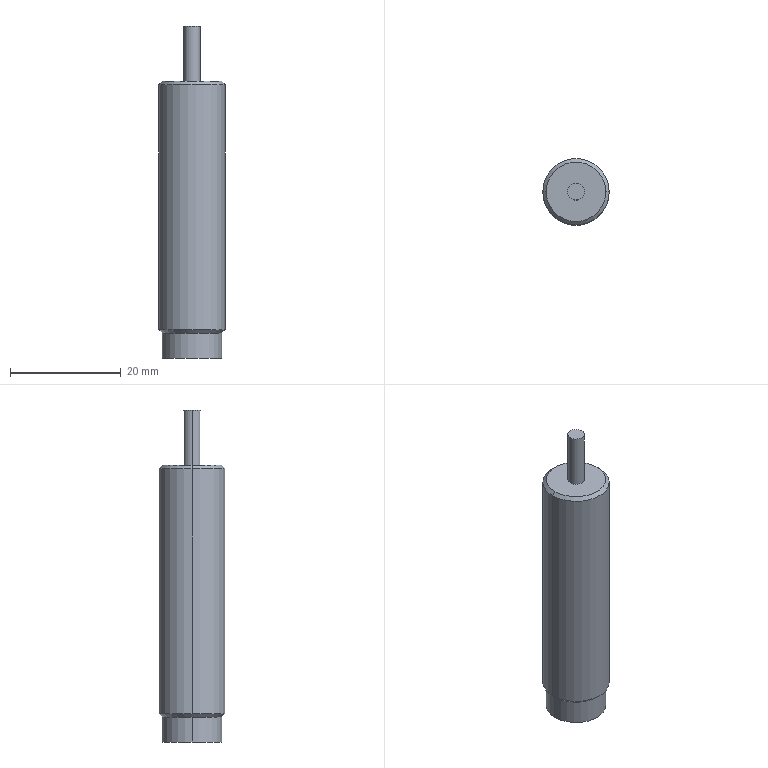Part | SolidWorks | features BaseBody 1 | 1 solid | 13 faces | box 12 x 12 x 60 mm | volume 5613 mm3 | cylinder 6 | cone 4 | plane 3 | commonest cylinder face diameters 3 x2 10.773 x2 12 x2
STEP:
#1=CARTESIAN_POINT('',(6.,0.,-44.886));
#2=VERTEX_POINT('',#1);
#3=CARTESIAN_POINT('',(-6.,0.,-44.886));
#4=VERTEX_POINT('',#3);
#5=CARTESIAN_POINT('',(0.,0.,-44.886));
#6=DIRECTION('',(0.,0.,1.));
#7=DIRECTION('',(1.,0.,0.));
#8=AXIS2_PLACEMENT_3D('',#5,#6,#7);
#9=CIRCLE('',#8,6.);
#10=EDGE_CURVE('',#2,#4,#9,.T.);
#11=ORIENTED_EDGE('',*,*,#10,.T.);
#12=CARTESIAN_POINT('',(-6.,0.,-0.6135));
#13=VERTEX_POINT('',#12);
#14=CARTESIAN_POINT('',(-6.,0.,-500.));
#15=DIRECTION('',(0.,0.,1.));
#16=VECTOR('',#15,1000.);
#17=LINE('',#14,#16);
#18=EDGE_CURVE('',#4,#13,#17,.T.);
#19=ORIENTED_EDGE('',*,*,#18,.T.);
#20=CARTESIAN_POINT('',(6.,0.,-0.6135));
#21=VERTEX_POINT('',#20);
#22=CARTESIAN_POINT('',(0.,0.,-0.6135));
#23=DIRECTION('',(0.,0.,-1.));
#24=DIRECTION('',(1.,0.,0.));
#25=AXIS2_PLACEMENT_3D('',#22,#23,#24);
#26=CIRCLE('',#25,6.);
#27=EDGE_CURVE('',#13,#21,#26,.T.);
#28=ORIENTED_EDGE('',*,*,#27,.T.);
#29=CARTESIAN_POINT('',(6.,0.,-500.));
#30=DIRECTION('',(0.,0.,1.));
#31=VECTOR('',#30,1000.);
#32=LINE('',#29,#31);
#33=EDGE_CURVE('',#2,#21,#32,.T.);
#34=ORIENTED_EDGE('',*,*,#33,.F.);
#35=EDGE_LOOP('',(#11,#19,#28,#34));
#36=FACE_OUTER_BOUND('',#35,.T.);
#37=CARTESIAN_POINT('',(0.,0.,-500.));
#38=DIRECTION('',(0.,0.,1.));
#39=DIRECTION('',(1.,0.,0.));
#40=AXIS2_PLACEMENT_3D('',#37,#38,#39);
#41=CYLINDRICAL_SURFACE('',#40,6.);
#42=ADVANCED_FACE('',(#36),#41,.T.);
#43=CARTESIAN_POINT('',(-5.386,0.,0.));
#44=VERTEX_POINT('',#43);
#45=CARTESIAN_POINT('',(5.386,0.,0.));
#46=VERTEX_POINT('',#45);
#47=CARTESIAN_POINT('',(0.,0.,0.));
#48=DIRECTION('',(0.,0.,-1.));
#49=DIRECTION('',(-1.,0.,0.));
#50=AXIS2_PLACEMENT_3D('',#47,#48,#49);
#51=CIRCLE('',#50,5.386);
#52=EDGE_CURVE('',#44,#46,#51,.T.);
#53=ORIENTED_EDGE('',*,*,#52,.T.);
#54=CARTESIAN_POINT('',(6.,0.,-0.6135));
#55=DIRECTION('',(0.7071,0.,-0.7071));
#56=VECTOR('',#55,1000.);
#57=LINE('',#54,#56);
#58=EDGE_CURVE('',#46,#21,#57,.T.);
#59=ORIENTED_EDGE('',*,*,#58,.T.);
#60=ORIENTED_EDGE('',*,*,#27,.F.);
#61=CARTESIAN_POINT('',(-6.,0.,-0.6135));
#62=DIRECTION('',(-0.7071,0.,-0.7071));
#63=VECTOR('',#62,1000.);
#64=LINE('',#61,#63);
#65=EDGE_CURVE('',#44,#13,#64,.T.);
#66=ORIENTED_EDGE('',*,*,#65,.F.);
#67=EDGE_LOOP('',(#53,#59,#60,#66));
#68=FACE_OUTER_BOUND('',#67,.T.);
#69=CARTESIAN_POINT('',(0.,0.,-0.6135));
#70=DIRECTION('',(0.,0.,-1.));
#71=DIRECTION('',(-1.,0.,0.));
#72=AXIS2_PLACEMENT_3D('',#69,#70,#71);
#73=CONICAL_SURFACE('',#72,6.,0.7854);
#74=ADVANCED_FACE('',(#68),#73,.T.);
#75=CARTESIAN_POINT('',(5.386,0.,-45.5));
#76=VERTEX_POINT('',#75);
#77=CARTESIAN_POINT('',(-5.386,0.,-45.5));
#78=VERTEX_POINT('',#77);
#79=CARTESIAN_POINT('',(0.,0.,-45.5));
#80=DIRECTION('',(0.,0.,1.));
#81=DIRECTION('',(1.,0.,0.));
#82=AXIS2_PLACEMENT_3D('',#79,#80,#81);
#83=CIRCLE('',#82,5.386);
#84=EDGE_CURVE('',#76,#78,#83,.T.);
#85=ORIENTED_EDGE('',*,*,#84,.T.);
#86=CARTESIAN_POINT('',(-6.,0.,-44.887));
#87=DIRECTION('',(-0.7071,0.,0.7071));
#88=VECTOR('',#87,1000.);
#89=LINE('',#86,#88);
#90=EDGE_CURVE('',#78,#4,#89,.T.);
#91=ORIENTED_EDGE('',*,*,#90,.T.);
#92=ORIENTED_EDGE('',*,*,#10,.F.);
#93=CARTESIAN_POINT('',(6.,0.,-44.887));
#94=DIRECTION('',(0.7071,0.,0.7071));
#95=VECTOR('',#94,1000.);
#96=LINE('',#93,#95);
#97=EDGE_CURVE('',#76,#2,#96,.T.);
#98=ORIENTED_EDGE('',*,*,#97,.F.);
#99=EDGE_LOOP('',(#85,#91,#92,#98));
#100=FACE_OUTER_BOUND('',#99,.T.);
#101=CARTESIAN_POINT('',(0.,0.,-44.887));
#102=DIRECTION('',(0.,0.,1.));
#103=DIRECTION('',(1.,0.,0.));
#104=AXIS2_PLACEMENT_3D('',#101,#102,#103);
#105=CONICAL_SURFACE('',#104,6.,0.7854);
#106=ADVANCED_FACE('',(#100),#105,.T.);
#107=CARTESIAN_POINT('',(5.387,0.,-50.));
#108=VERTEX_POINT('',#107);
#109=CARTESIAN_POINT('',(-5.387,0.,-50.));
#110=VERTEX_POINT('',#109);
#111=CARTESIAN_POINT('',(0.,0.,-50.));
#112=DIRECTION('',(0.,0.,1.));
#113=DIRECTION('',(1.,0.,0.));
#114=AXIS2_PLACEMENT_3D('',#111,#112,#113);
#115=CIRCLE('',#114,5.387);
#116=EDGE_CURVE('',#108,#110,#115,.T.);
#117=ORIENTED_EDGE('',*,*,#116,.T.);
#118=CARTESIAN_POINT('',(-5.387,0.,-500.));
#119=DIRECTION('',(0.,0.,1.));
#120=VECTOR('',#119,1000.);
#121=LINE('',#118,#120);
#122=EDGE_CURVE('',#110,#78,#121,.T.);
#123=ORIENTED_EDGE('',*,*,#122,.T.);
#124=ORIENTED_EDGE('',*,*,#84,.F.);
#125=CARTESIAN_POINT('',(5.387,0.,-500.));
#126=DIRECTION('',(0.,0.,1.));
#127=VECTOR('',#126,1000.);
#128=LINE('',#125,#127);
#129=EDGE_CURVE('',#108,#76,#128,.T.);
#130=ORIENTED_EDGE('',*,*,#129,.F.);
#131=EDGE_LOOP('',(#117,#123,#124,#130));
#132=FACE_OUTER_BOUND('',#131,.T.);
#133=CARTESIAN_POINT('',(0.,0.,-500.));
#134=DIRECTION('',(0.,0.,1.));
#135=DIRECTION('',(1.,0.,0.));
#136=AXIS2_PLACEMENT_3D('',#133,#134,#135);
#137=CYLINDRICAL_SURFACE('',#136,5.387);
#138=ADVANCED_FACE('',(#132),#137,.T.);
#139=CARTESIAN_POINT('',(1.5,0.,0.));
#140=VERTEX_POINT('',#139);
#141=CARTESIAN_POINT('',(-1.5,0.,0.));
#142=VERTEX_POINT('',#141);
#143=CARTESIAN_POINT('',(0.,0.,0.));
#144=DIRECTION('',(0.,0.,1.));
#145=DIRECTION('',(1.,0.,0.));
#146=AXIS2_PLACEMENT_3D('',#143,#144,#145);
#147=CIRCLE('',#146,1.5);
#148=EDGE_CURVE('',#140,#142,#147,.T.);
#149=ORIENTED_EDGE('',*,*,#148,.T.);
#150=CARTESIAN_POINT('',(-1.5,0.,10.));
#151=VERTEX_POINT('',#150);
#152=CARTESIAN_POINT('',(-1.5,0.,-500.));
#153=DIRECTION('',(0.,0.,1.));
#154=VECTOR('',#153,1000.);
#155=LINE('',#152,#154);
#156=EDGE_CURVE('',#142,#151,#155,.T.);
#157=ORIENTED_EDGE('',*,*,#156,.T.);
#158=CARTESIAN_POINT('',(1.5,0.,10.));
#159=VERTEX_POINT('',#158);
#160=CARTESIAN_POINT('',(0.,0.,10.));
#161=DIRECTION('',(0.,0.,-1.));
#162=DIRECTION('',(1.,0.,0.));
#163=AXIS2_PLACEMENT_3D('',#160,#161,#162);
#164=CIRCLE('',#163,1.5);
#165=EDGE_CURVE('',#151,#159,#164,.T.);
#166=ORIENTED_EDGE('',*,*,#165,.T.);
#167=CARTESIAN_POINT('',(1.5,0.,-500.));
#168=DIRECTION('',(0.,0.,1.));
#169=VECTOR('',#168,1000.);
#170=LINE('',#167,#169);
#171=EDGE_CURVE('',#140,#159,#170,.T.);
#172=ORIENTED_EDGE('',*,*,#171,.F.);
#173=EDGE_LOOP('',(#149,#157,#166,#172));
#174=FACE_OUTER_BOUND('',#173,.T.);
#175=CARTESIAN_POINT('',(0.,0.,-500.));
#176=DIRECTION('',(0.,0.,1.));
#177=DIRECTION('',(1.,0.,0.));
#178=AXIS2_PLACEMENT_3D('',#175,#176,#177);
#179=CYLINDRICAL_SURFACE('',#178,1.5);
#180=ADVANCED_FACE('',(#174),#179,.T.);
#181=ORIENTED_EDGE('',*,*,#18,.F.);
#182=CARTESIAN_POINT('',(0.,0.,-44.886));
#183=DIRECTION('',(0.,0.,1.));
#184=DIRECTION('',(1.,0.,0.));
#185=AXIS2_PLACEMENT_3D('',#182,#183,#184);
#186=CIRCLE('',#185,6.);
#187=EDGE_CURVE('',#4,#2,#186,.T.);
#188=ORIENTED_EDGE('',*,*,#187,.T.);
#189=ORIENTED_EDGE('',*,*,#33,.T.);
#190=CARTESIAN_POINT('',(0.,0.,-0.6135));
#191=DIRECTION('',(0.,0.,-1.));
#192=DIRECTION('',(1.,0.,0.));
#193=AXIS2_PLACEMENT_3D('',#190,#191,#192);
#194=CIRCLE('',#193,6.);
#195=EDGE_CURVE('',#21,#13,#194,.T.);
#196=ORIENTED_EDGE('',*,*,#195,.T.);
#197=EDGE_LOOP('',(#181,#188,#189,#196));
#198=FACE_OUTER_BOUND('',#197,.T.);
#199=CARTESIAN_POINT('',(0.,0.,-500.));
#200=DIRECTION('',(0.,0.,1.));
#201=DIRECTION('',(1.,0.,0.));
#202=AXIS2_PLACEMENT_3D('',#199,#200,#201);
#203=CYLINDRICAL_SURFACE('',#202,6.);
#204=ADVANCED_FACE('',(#198),#203,.T.);
#205=ORIENTED_EDGE('',*,*,#58,.F.);
#206=CARTESIAN_POINT('',(0.,0.,0.));
#207=DIRECTION('',(0.,0.,-1.));
#208=DIRECTION('',(-1.,0.,0.));
#209=AXIS2_PLACEMENT_3D('',#206,#207,#208);
#210=CIRCLE('',#209,5.386);
#211=EDGE_CURVE('',#46,#44,#210,.T.);
#212=ORIENTED_EDGE('',*,*,#211,.T.);
#213=ORIENTED_EDGE('',*,*,#65,.T.);
#214=ORIENTED_EDGE('',*,*,#195,.F.);
#215=EDGE_LOOP('',(#205,#212,#213,#214));
#216=FACE_OUTER_BOUND('',#215,.T.);
#217=CARTESIAN_POINT('',(0.,0.,-0.6135));
#218=DIRECTION('',(0.,0.,-1.));
#219=DIRECTION('',(-1.,0.,0.));
#220=AXIS2_PLACEMENT_3D('',#217,#218,#219);
#221=CONICAL_SURFACE('',#220,6.,0.7854);
#222=ADVANCED_FACE('',(#216),#221,.T.);
#223=ORIENTED_EDGE('',*,*,#90,.F.);
#224=CARTESIAN_POINT('',(0.,0.,-45.5));
#225=DIRECTION('',(0.,0.,1.));
#226=DIRECTION('',(1.,0.,0.));
#227=AXIS2_PLACEMENT_3D('',#224,#225,#226);
#228=CIRCLE('',#227,5.386);
#229=EDGE_CURVE('',#78,#76,#228,.T.);
#230=ORIENTED_EDGE('',*,*,#229,.T.);
#231=ORIENTED_EDGE('',*,*,#97,.T.);
#232=ORIENTED_EDGE('',*,*,#187,.F.);
#233=EDGE_LOOP('',(#223,#230,#231,#232));
#234=FACE_OUTER_BOUND('',#233,.T.);
#235=CARTESIAN_POINT('',(0.,0.,-44.887));
#236=DIRECTION('',(0.,0.,1.));
#237=DIRECTION('',(1.,0.,0.));
#238=AXIS2_PLACEMENT_3D('',#235,#236,#237);
#239=CONICAL_SURFACE('',#238,6.,0.7854);
#240=ADVANCED_FACE('',(#234),#239,.T.);
#241=ORIENTED_EDGE('',*,*,#148,.F.);
#242=CARTESIAN_POINT('',(0.,0.,0.));
#243=DIRECTION('',(0.,0.,1.));
#244=DIRECTION('',(1.,0.,0.));
#245=AXIS2_PLACEMENT_3D('',#242,#243,#244);
#246=CIRCLE('',#245,1.5);
#247=EDGE_CURVE('',#142,#140,#246,.T.);
#248=ORIENTED_EDGE('',*,*,#247,.F.);
#249=EDGE_LOOP('',(#241,#248));
#250=FACE_BOUND('',#249,.T.);
#251=ORIENTED_EDGE('',*,*,#52,.F.);
#252=ORIENTED_EDGE('',*,*,#211,.F.);
#253=EDGE_LOOP('',(#251,#252));
#254=FACE_OUTER_BOUND('',#253,.T.);
#255=CARTESIAN_POINT('',(0.,1.5,0.));
#256=DIRECTION('',(0.,0.,-1.));
#257=DIRECTION('',(-1.,0.,0.));
#258=AXIS2_PLACEMENT_3D('',#255,#256,#257);
#259=PLANE('',#258);
#260=ADVANCED_FACE('',(#250,#254),#259,.F.);
#261=ORIENTED_EDGE('',*,*,#122,.F.);
#262=CARTESIAN_POINT('',(0.,0.,-50.));
#263=DIRECTION('',(0.,0.,1.));
#264=DIRECTION('',(1.,0.,0.));
#265=AXIS2_PLACEMENT_3D('',#262,#263,#264);
#266=CIRCLE('',#265,5.387);
#267=EDGE_CURVE('',#110,#108,#266,.T.);
#268=ORIENTED_EDGE('',*,*,#267,.T.);
#269=ORIENTED_EDGE('',*,*,#129,.T.);
#270=ORIENTED_EDGE('',*,*,#229,.F.);
#271=EDGE_LOOP('',(#261,#268,#269,#270));
#272=FACE_OUTER_BOUND('',#271,.T.);
#273=CARTESIAN_POINT('',(0.,0.,-500.));
#274=DIRECTION('',(0.,0.,1.));
#275=DIRECTION('',(1.,0.,0.));
#276=AXIS2_PLACEMENT_3D('',#273,#274,#275);
#277=CYLINDRICAL_SURFACE('',#276,5.387);
#278=ADVANCED_FACE('',(#272),#277,.T.);
#279=ORIENTED_EDGE('',*,*,#156,.F.);
#280=ORIENTED_EDGE('',*,*,#247,.T.);
#281=ORIENTED_EDGE('',*,*,#171,.T.);
#282=CARTESIAN_POINT('',(0.,0.,10.));
#283=DIRECTION('',(0.,0.,-1.));
#284=DIRECTION('',(1.,0.,0.));
#285=AXIS2_PLACEMENT_3D('',#282,#283,#284);
#286=CIRCLE('',#285,1.5);
#287=EDGE_CURVE('',#159,#151,#286,.T.);
#288=ORIENTED_EDGE('',*,*,#287,.T.);
#289=EDGE_LOOP('',(#279,#280,#281,#288));
#290=FACE_OUTER_BOUND('',#289,.T.);
#291=CARTESIAN_POINT('',(0.,0.,-500.));
#292=DIRECTION('',(0.,0.,1.));
#293=DIRECTION('',(1.,0.,0.));
#294=AXIS2_PLACEMENT_3D('',#291,#292,#293);
#295=CYLINDRICAL_SURFACE('',#294,1.5);
#296=ADVANCED_FACE('',(#290),#295,.T.);
#297=ORIENTED_EDGE('',*,*,#116,.F.);
#298=ORIENTED_EDGE('',*,*,#267,.F.);
#299=EDGE_LOOP('',(#297,#298));
#300=FACE_OUTER_BOUND('',#299,.T.);
#301=CARTESIAN_POINT('',(0.,5.387,-50.));
#302=DIRECTION('',(0.,0.,1.));
#303=DIRECTION('',(1.,0.,0.));
#304=AXIS2_PLACEMENT_3D('',#301,#302,#303);
#305=PLANE('',#304);
#306=ADVANCED_FACE('',(#300),#305,.F.);
#307=ORIENTED_EDGE('',*,*,#287,.F.);
#308=ORIENTED_EDGE('',*,*,#165,.F.);
#309=EDGE_LOOP('',(#307,#308));
#310=FACE_OUTER_BOUND('',#309,.T.);
#311=CARTESIAN_POINT('',(0.,0.,10.));
#312=DIRECTION('',(0.,0.,-1.));
#313=DIRECTION('',(-1.,0.,0.));
#314=AXIS2_PLACEMENT_3D('',#311,#312,#313);
#315=PLANE('',#314);
#316=ADVANCED_FACE('',(#310),#315,.F.);
#317=CLOSED_SHELL('',(#42,#74,#106,#138,#180,#204,#222,#240,#260,#278,#296,#306,#316));
#318=MANIFOLD_SOLID_BREP('',#317);
#319=CARTESIAN_POINT('',(0.,0.,0.));
#320=DIRECTION('',(0.,0.,1.));
#321=DIRECTION('',(1.,0.,0.));
#322=AXIS2_PLACEMENT_3D('',#319,#320,#321);
#323=(LENGTH_UNIT()NAMED_UNIT(*)SI_UNIT(.MILLI.,.METRE.));
#324=UNCERTAINTY_MEASURE_WITH_UNIT(LENGTH_MEASURE(0.00001),#323,'','');
#325=(NAMED_UNIT(*)PLANE_ANGLE_UNIT()SI_UNIT($,.RADIAN.));
#326=(NAMED_UNIT(*)SI_UNIT($,.STERADIAN.)SOLID_ANGLE_UNIT());
#327=(GEOMETRIC_REPRESENTATION_CONTEXT(3)GLOBAL_UNCERTAINTY_ASSIGNED_CONTEXT((#324))GLOBAL_UNIT_ASSIGNED_CONTEXT((#323,#325,#326))REPRESENTATION_CONTEXT('',''));
#328=ADVANCED_BREP_SHAPE_REPRESENTATION('',(#318,#322),#327);